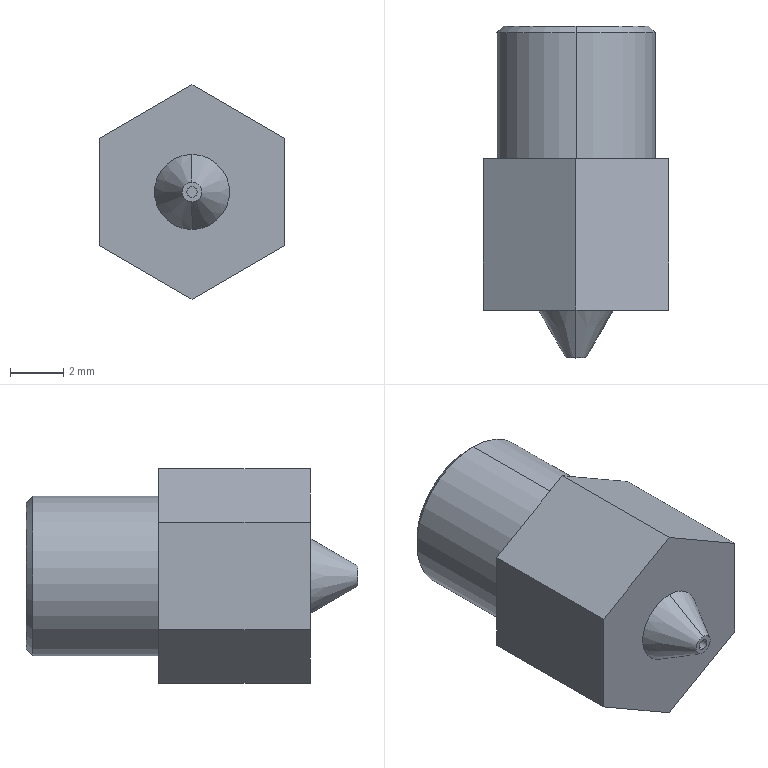Part | SolidWorks | features ICE 1, Revolution 1 | 1 solid | 28 faces | box 7 x 12.5 x 8.083 mm | volume 370.688 mm3 | plane 12 | cylinder 8 | cone 8 | commonest cylinder face diameters 0.4 x2 1 x2 2 x2 6 x2
STEP:
#1=CARTESIAN_POINT('',(0.,12.,1.));
#2=VERTEX_POINT('',#1);
#3=CARTESIAN_POINT('',(0.,12.,-1.));
#4=VERTEX_POINT('',#3);
#5=CARTESIAN_POINT('',(0.,12.,0.));
#6=DIRECTION('',(0.,-1.,0.));
#7=DIRECTION('',(0.,0.,-1.));
#8=AXIS2_PLACEMENT_3D('',#5,#6,#7);
#9=CIRCLE('',#8,1.);
#10=EDGE_CURVE('',#2,#4,#9,.T.);
#11=ORIENTED_EDGE('',*,*,#10,.F.);
#12=CARTESIAN_POINT('',(0.,7.5,1.));
#13=VERTEX_POINT('',#12);
#14=CARTESIAN_POINT('',(0.,0.,1.));
#15=DIRECTION('',(0.,-1.,0.));
#16=VECTOR('',#15,1000.);
#17=LINE('',#14,#16);
#18=EDGE_CURVE('',#2,#13,#17,.T.);
#19=ORIENTED_EDGE('',*,*,#18,.T.);
#20=CARTESIAN_POINT('',(0.,7.5,-1.));
#21=VERTEX_POINT('',#20);
#22=CARTESIAN_POINT('',(0.,7.5,0.));
#23=DIRECTION('',(0.,1.,0.));
#24=DIRECTION('',(0.,0.,1.));
#25=AXIS2_PLACEMENT_3D('',#22,#23,#24);
#26=CIRCLE('',#25,1.);
#27=EDGE_CURVE('',#21,#13,#26,.T.);
#28=ORIENTED_EDGE('',*,*,#27,.F.);
#29=CARTESIAN_POINT('',(0.,0.,-1.));
#30=DIRECTION('',(0.,-1.,0.));
#31=VECTOR('',#30,1000.);
#32=LINE('',#29,#31);
#33=EDGE_CURVE('',#4,#21,#32,.T.);
#34=ORIENTED_EDGE('',*,*,#33,.F.);
#35=EDGE_LOOP('',(#11,#19,#28,#34));
#36=FACE_OUTER_BOUND('',#35,.T.);
#37=CARTESIAN_POINT('',(0.,0.,0.));
#38=DIRECTION('',(0.,-1.,0.));
#39=DIRECTION('',(0.,0.,-1.));
#40=AXIS2_PLACEMENT_3D('',#37,#38,#39);
#41=CYLINDRICAL_SURFACE('',#40,1.);
#42=ADVANCED_FACE('',(#36),#41,.F.);
#43=ORIENTED_EDGE('',*,*,#10,.T.);
#44=CARTESIAN_POINT('',(0.,12.5,-1.289));
#45=VERTEX_POINT('',#44);
#46=CARTESIAN_POINT('',(0.,12.5,-1.289));
#47=DIRECTION('',(0.,0.866,-0.5));
#48=VECTOR('',#47,1000.);
#49=LINE('',#46,#48);
#50=EDGE_CURVE('',#4,#45,#49,.T.);
#51=ORIENTED_EDGE('',*,*,#50,.T.);
#52=CARTESIAN_POINT('',(0.,12.5,1.289));
#53=VERTEX_POINT('',#52);
#54=CARTESIAN_POINT('',(0.,12.5,0.));
#55=DIRECTION('',(0.,-1.,0.));
#56=DIRECTION('',(0.,0.,-1.));
#57=AXIS2_PLACEMENT_3D('',#54,#55,#56);
#58=CIRCLE('',#57,1.289);
#59=EDGE_CURVE('',#53,#45,#58,.T.);
#60=ORIENTED_EDGE('',*,*,#59,.F.);
#61=CARTESIAN_POINT('',(0.,12.5,1.289));
#62=DIRECTION('',(0.,0.866,0.5));
#63=VECTOR('',#62,1000.);
#64=LINE('',#61,#63);
#65=EDGE_CURVE('',#2,#53,#64,.T.);
#66=ORIENTED_EDGE('',*,*,#65,.F.);
#67=EDGE_LOOP('',(#43,#51,#60,#66));
#68=FACE_OUTER_BOUND('',#67,.T.);
#69=CARTESIAN_POINT('',(0.,12.5,0.));
#70=DIRECTION('',(0.,1.,0.));
#71=DIRECTION('',(0.,0.,1.));
#72=AXIS2_PLACEMENT_3D('',#69,#70,#71);
#73=CONICAL_SURFACE('',#72,1.289,0.5236);
#74=ADVANCED_FACE('',(#68),#73,.F.);
#75=CARTESIAN_POINT('',(0.,12.25,-3.));
#76=VERTEX_POINT('',#75);
#77=CARTESIAN_POINT('',(0.,12.25,3.));
#78=VERTEX_POINT('',#77);
#79=CARTESIAN_POINT('',(0.,12.25,0.));
#80=DIRECTION('',(0.,-1.,0.));
#81=DIRECTION('',(0.,0.,-1.));
#82=AXIS2_PLACEMENT_3D('',#79,#80,#81);
#83=CIRCLE('',#82,3.);
#84=EDGE_CURVE('',#76,#78,#83,.T.);
#85=ORIENTED_EDGE('',*,*,#84,.T.);
#86=CARTESIAN_POINT('',(0.,7.5,3.));
#87=VERTEX_POINT('',#86);
#88=CARTESIAN_POINT('',(0.,0.,3.));
#89=DIRECTION('',(0.,-1.,0.));
#90=VECTOR('',#89,1000.);
#91=LINE('',#88,#90);
#92=EDGE_CURVE('',#78,#87,#91,.T.);
#93=ORIENTED_EDGE('',*,*,#92,.T.);
#94=CARTESIAN_POINT('',(0.,7.5,-3.));
#95=VERTEX_POINT('',#94);
#96=CARTESIAN_POINT('',(0.,7.5,0.));
#97=DIRECTION('',(0.,-1.,0.));
#98=DIRECTION('',(0.,0.,1.));
#99=AXIS2_PLACEMENT_3D('',#96,#97,#98);
#100=CIRCLE('',#99,3.);
#101=EDGE_CURVE('',#95,#87,#100,.T.);
#102=ORIENTED_EDGE('',*,*,#101,.F.);
#103=CARTESIAN_POINT('',(0.,0.,-3.));
#104=DIRECTION('',(0.,-1.,0.));
#105=VECTOR('',#104,1000.);
#106=LINE('',#103,#105);
#107=EDGE_CURVE('',#76,#95,#106,.T.);
#108=ORIENTED_EDGE('',*,*,#107,.F.);
#109=EDGE_LOOP('',(#85,#93,#102,#108));
#110=FACE_OUTER_BOUND('',#109,.T.);
#111=CARTESIAN_POINT('',(0.,0.,0.));
#112=DIRECTION('',(0.,-1.,0.));
#113=DIRECTION('',(0.,0.,-1.));
#114=AXIS2_PLACEMENT_3D('',#111,#112,#113);
#115=CYLINDRICAL_SURFACE('',#114,3.);
#116=ADVANCED_FACE('',(#110),#115,.T.);
#117=CARTESIAN_POINT('',(0.,12.5,-2.75));
#118=VERTEX_POINT('',#117);
#119=CARTESIAN_POINT('',(0.,12.5,2.75));
#120=VERTEX_POINT('',#119);
#121=CARTESIAN_POINT('',(0.,12.5,0.));
#122=DIRECTION('',(0.,-1.,0.));
#123=DIRECTION('',(0.,0.,-1.));
#124=AXIS2_PLACEMENT_3D('',#121,#122,#123);
#125=CIRCLE('',#124,2.75);
#126=EDGE_CURVE('',#118,#120,#125,.T.);
#127=ORIENTED_EDGE('',*,*,#126,.T.);
#128=CARTESIAN_POINT('',(0.,12.25,3.));
#129=DIRECTION('',(0.,-0.7071,0.7071));
#130=VECTOR('',#129,1000.);
#131=LINE('',#128,#130);
#132=EDGE_CURVE('',#120,#78,#131,.T.);
#133=ORIENTED_EDGE('',*,*,#132,.T.);
#134=ORIENTED_EDGE('',*,*,#84,.F.);
#135=CARTESIAN_POINT('',(0.,12.25,-3.));
#136=DIRECTION('',(0.,-0.7071,-0.7071));
#137=VECTOR('',#136,1000.);
#138=LINE('',#135,#137);
#139=EDGE_CURVE('',#118,#76,#138,.T.);
#140=ORIENTED_EDGE('',*,*,#139,.F.);
#141=EDGE_LOOP('',(#127,#133,#134,#140));
#142=FACE_OUTER_BOUND('',#141,.T.);
#143=CARTESIAN_POINT('',(0.,12.25,0.));
#144=DIRECTION('',(0.,-1.,0.));
#145=DIRECTION('',(0.,0.,-1.));
#146=AXIS2_PLACEMENT_3D('',#143,#144,#145);
#147=CONICAL_SURFACE('',#146,3.,0.7854);
#148=ADVANCED_FACE('',(#142),#147,.T.);
#149=CARTESIAN_POINT('',(0.,0.6,0.2));
#150=VERTEX_POINT('',#149);
#151=CARTESIAN_POINT('',(0.,0.6,-0.2));
#152=VERTEX_POINT('',#151);
#153=CARTESIAN_POINT('',(0.,0.6,0.));
#154=DIRECTION('',(0.,-1.,0.));
#155=DIRECTION('',(0.,0.,-1.));
#156=AXIS2_PLACEMENT_3D('',#153,#154,#155);
#157=CIRCLE('',#156,0.2);
#158=EDGE_CURVE('',#150,#152,#157,.T.);
#159=ORIENTED_EDGE('',*,*,#158,.F.);
#160=CARTESIAN_POINT('',(0.,0.,0.2));
#161=VERTEX_POINT('',#160);
#162=CARTESIAN_POINT('',(0.,0.,0.2));
#163=DIRECTION('',(0.,-1.,0.));
#164=VECTOR('',#163,1000.);
#165=LINE('',#162,#164);
#166=EDGE_CURVE('',#150,#161,#165,.T.);
#167=ORIENTED_EDGE('',*,*,#166,.T.);
#168=CARTESIAN_POINT('',(0.,0.,-0.2));
#169=VERTEX_POINT('',#168);
#170=CARTESIAN_POINT('',(0.,0.,0.));
#171=DIRECTION('',(0.,-1.,0.));
#172=DIRECTION('',(0.,0.,-1.));
#173=AXIS2_PLACEMENT_3D('',#170,#171,#172);
#174=CIRCLE('',#173,0.2);
#175=EDGE_CURVE('',#161,#169,#174,.T.);
#176=ORIENTED_EDGE('',*,*,#175,.T.);
#177=CARTESIAN_POINT('',(0.,0.,-0.2));
#178=DIRECTION('',(0.,-1.,0.));
#179=VECTOR('',#178,1000.);
#180=LINE('',#177,#179);
#181=EDGE_CURVE('',#152,#169,#180,.T.);
#182=ORIENTED_EDGE('',*,*,#181,.F.);
#183=EDGE_LOOP('',(#159,#167,#176,#182));
#184=FACE_OUTER_BOUND('',#183,.T.);
#185=CARTESIAN_POINT('',(0.,0.,0.));
#186=DIRECTION('',(0.,-1.,0.));
#187=DIRECTION('',(0.,0.,-1.));
#188=AXIS2_PLACEMENT_3D('',#185,#186,#187);
#189=CYLINDRICAL_SURFACE('',#188,0.2);
#190=ADVANCED_FACE('',(#184),#189,.F.);
#191=ORIENTED_EDGE('',*,*,#158,.T.);
#192=CARTESIAN_POINT('',(0.,1.12,-0.5));
#193=VERTEX_POINT('',#192);
#194=CARTESIAN_POINT('',(0.,1.12,-0.5));
#195=DIRECTION('',(0.,0.866,-0.5));
#196=VECTOR('',#195,1000.);
#197=LINE('',#194,#196);
#198=EDGE_CURVE('',#152,#193,#197,.T.);
#199=ORIENTED_EDGE('',*,*,#198,.T.);
#200=CARTESIAN_POINT('',(0.,1.12,0.5));
#201=VERTEX_POINT('',#200);
#202=CARTESIAN_POINT('',(0.,1.12,0.));
#203=DIRECTION('',(0.,-1.,0.));
#204=DIRECTION('',(0.,0.,-1.));
#205=AXIS2_PLACEMENT_3D('',#202,#203,#204);
#206=CIRCLE('',#205,0.5);
#207=EDGE_CURVE('',#201,#193,#206,.T.);
#208=ORIENTED_EDGE('',*,*,#207,.F.);
#209=CARTESIAN_POINT('',(0.,1.12,0.5));
#210=DIRECTION('',(0.,0.866,0.5));
#211=VECTOR('',#210,1000.);
#212=LINE('',#209,#211);
#213=EDGE_CURVE('',#150,#201,#212,.T.);
#214=ORIENTED_EDGE('',*,*,#213,.F.);
#215=EDGE_LOOP('',(#191,#199,#208,#214));
#216=FACE_OUTER_BOUND('',#215,.T.);
#217=CARTESIAN_POINT('',(0.,1.12,0.));
#218=DIRECTION('',(0.,1.,0.));
#219=DIRECTION('',(0.,0.,1.));
#220=AXIS2_PLACEMENT_3D('',#217,#218,#219);
#221=CONICAL_SURFACE('',#220,0.5,0.5236);
#222=ADVANCED_FACE('',(#216),#221,.F.);
#223=CARTESIAN_POINT('',(0.,1.8,0.5));
#224=VERTEX_POINT('',#223);
#225=CARTESIAN_POINT('',(0.,1.8,-0.5));
#226=VERTEX_POINT('',#225);
#227=CARTESIAN_POINT('',(0.,1.8,0.));
#228=DIRECTION('',(0.,-1.,0.));
#229=DIRECTION('',(0.,0.,-1.));
#230=AXIS2_PLACEMENT_3D('',#227,#228,#229);
#231=CIRCLE('',#230,0.5);
#232=EDGE_CURVE('',#224,#226,#231,.T.);
#233=ORIENTED_EDGE('',*,*,#232,.F.);
#234=CARTESIAN_POINT('',(0.,0.,0.5));
#235=DIRECTION('',(0.,-1.,0.));
#236=VECTOR('',#235,1000.);
#237=LINE('',#234,#236);
#238=EDGE_CURVE('',#224,#201,#237,.T.);
#239=ORIENTED_EDGE('',*,*,#238,.T.);
#240=ORIENTED_EDGE('',*,*,#207,.T.);
#241=CARTESIAN_POINT('',(0.,0.,-0.5));
#242=DIRECTION('',(0.,-1.,0.));
#243=VECTOR('',#242,1000.);
#244=LINE('',#241,#243);
#245=EDGE_CURVE('',#226,#193,#244,.T.);
#246=ORIENTED_EDGE('',*,*,#245,.F.);
#247=EDGE_LOOP('',(#233,#239,#240,#246));
#248=FACE_OUTER_BOUND('',#247,.T.);
#249=CARTESIAN_POINT('',(0.,0.,0.));
#250=DIRECTION('',(0.,-1.,0.));
#251=DIRECTION('',(0.,0.,-1.));
#252=AXIS2_PLACEMENT_3D('',#249,#250,#251);
#253=CYLINDRICAL_SURFACE('',#252,0.5);
#254=ADVANCED_FACE('',(#248),#253,.F.);
#255=CARTESIAN_POINT('',(0.,0.,-0.375));
#256=VERTEX_POINT('',#255);
#257=CARTESIAN_POINT('',(0.,0.,0.375));
#258=VERTEX_POINT('',#257);
#259=CARTESIAN_POINT('',(0.,0.,0.));
#260=DIRECTION('',(0.,-1.,0.));
#261=DIRECTION('',(0.,0.,-1.));
#262=AXIS2_PLACEMENT_3D('',#259,#260,#261);
#263=CIRCLE('',#262,0.375);
#264=EDGE_CURVE('',#256,#258,#263,.T.);
#265=ORIENTED_EDGE('',*,*,#264,.F.);
#266=CARTESIAN_POINT('',(0.,1.8,-1.414));
#267=VERTEX_POINT('',#266);
#268=CARTESIAN_POINT('',(0.,0.,-0.375));
#269=DIRECTION('',(0.,0.866,-0.5));
#270=VECTOR('',#269,1000.);
#271=LINE('',#268,#270);
#272=EDGE_CURVE('',#256,#267,#271,.T.);
#273=ORIENTED_EDGE('',*,*,#272,.T.);
#274=CARTESIAN_POINT('',(0.,1.8,1.414));
#275=VERTEX_POINT('',#274);
#276=CARTESIAN_POINT('',(0.,1.8,0.));
#277=DIRECTION('',(0.,-1.,0.));
#278=DIRECTION('',(0.,0.,-1.));
#279=AXIS2_PLACEMENT_3D('',#276,#277,#278);
#280=CIRCLE('',#279,1.414);
#281=EDGE_CURVE('',#267,#275,#280,.T.);
#282=ORIENTED_EDGE('',*,*,#281,.T.);
#283=CARTESIAN_POINT('',(0.,0.,0.375));
#284=DIRECTION('',(0.,0.866,0.5));
#285=VECTOR('',#284,1000.);
#286=LINE('',#283,#285);
#287=EDGE_CURVE('',#258,#275,#286,.T.);
#288=ORIENTED_EDGE('',*,*,#287,.F.);
#289=EDGE_LOOP('',(#265,#273,#282,#288));
#290=FACE_OUTER_BOUND('',#289,.T.);
#291=CARTESIAN_POINT('',(0.,0.,0.));
#292=DIRECTION('',(0.,1.,0.));
#293=DIRECTION('',(0.,0.,1.));
#294=AXIS2_PLACEMENT_3D('',#291,#292,#293);
#295=CONICAL_SURFACE('',#294,0.375,0.5236);
#296=ADVANCED_FACE('',(#290),#295,.T.);
#297=ORIENTED_EDGE('',*,*,#272,.F.);
#298=CARTESIAN_POINT('',(0.,0.,0.));
#299=DIRECTION('',(0.,-1.,0.));
#300=DIRECTION('',(0.,0.,-1.));
#301=AXIS2_PLACEMENT_3D('',#298,#299,#300);
#302=CIRCLE('',#301,0.375);
#303=EDGE_CURVE('',#258,#256,#302,.T.);
#304=ORIENTED_EDGE('',*,*,#303,.F.);
#305=ORIENTED_EDGE('',*,*,#287,.T.);
#306=CARTESIAN_POINT('',(0.,1.8,0.));
#307=DIRECTION('',(0.,-1.,0.));
#308=DIRECTION('',(0.,0.,-1.));
#309=AXIS2_PLACEMENT_3D('',#306,#307,#308);
#310=CIRCLE('',#309,1.414);
#311=EDGE_CURVE('',#275,#267,#310,.T.);
#312=ORIENTED_EDGE('',*,*,#311,.T.);
#313=EDGE_LOOP('',(#297,#304,#305,#312));
#314=FACE_OUTER_BOUND('',#313,.T.);
#315=CARTESIAN_POINT('',(0.,0.,0.));
#316=DIRECTION('',(0.,1.,0.));
#317=DIRECTION('',(0.,0.,1.));
#318=AXIS2_PLACEMENT_3D('',#315,#316,#317);
#319=CONICAL_SURFACE('',#318,0.375,0.5236);
#320=ADVANCED_FACE('',(#314),#319,.T.);
#321=ORIENTED_EDGE('',*,*,#311,.F.);
#322=ORIENTED_EDGE('',*,*,#281,.F.);
#323=EDGE_LOOP('',(#321,#322));
#324=FACE_BOUND('',#323,.T.);
#325=CARTESIAN_POINT('',(3.5,1.8,2.021));
#326=VERTEX_POINT('',#325);
#327=CARTESIAN_POINT('',(0.,1.8,4.041));
#328=VERTEX_POINT('',#327);
#329=CARTESIAN_POINT('',(3.5,1.8,2.021));
#330=DIRECTION('',(-0.866,0.,0.5));
#331=VECTOR('',#330,1000.);
#332=LINE('',#329,#331);
#333=EDGE_CURVE('',#326,#328,#332,.T.);
#334=ORIENTED_EDGE('',*,*,#333,.T.);
#335=CARTESIAN_POINT('',(-3.5,1.8,2.021));
#336=VERTEX_POINT('',#335);
#337=CARTESIAN_POINT('',(0.,1.8,4.041));
#338=DIRECTION('',(-0.866,0.,-0.5));
#339=VECTOR('',#338,1000.);
#340=LINE('',#337,#339);
#341=EDGE_CURVE('',#328,#336,#340,.T.);
#342=ORIENTED_EDGE('',*,*,#341,.T.);
#343=CARTESIAN_POINT('',(-3.5,1.8,-2.021));
#344=VERTEX_POINT('',#343);
#345=CARTESIAN_POINT('',(-3.5,1.8,2.021));
#346=DIRECTION('',(0.,0.,-1.));
#347=VECTOR('',#346,1000.);
#348=LINE('',#345,#347);
#349=EDGE_CURVE('',#336,#344,#348,.T.);
#350=ORIENTED_EDGE('',*,*,#349,.T.);
#351=CARTESIAN_POINT('',(0.,1.8,-4.041));
#352=VERTEX_POINT('',#351);
#353=CARTESIAN_POINT('',(-3.5,1.8,-2.021));
#354=DIRECTION('',(0.866,0.,-0.5));
#355=VECTOR('',#354,1000.);
#356=LINE('',#353,#355);
#357=EDGE_CURVE('',#344,#352,#356,.T.);
#358=ORIENTED_EDGE('',*,*,#357,.T.);
#359=CARTESIAN_POINT('',(3.5,1.8,-2.021));
#360=VERTEX_POINT('',#359);
#361=CARTESIAN_POINT('',(0.,1.8,-4.041));
#362=DIRECTION('',(0.866,0.,0.5));
#363=VECTOR('',#362,1000.);
#364=LINE('',#361,#363);
#365=EDGE_CURVE('',#352,#360,#364,.T.);
#366=ORIENTED_EDGE('',*,*,#365,.T.);
#367=CARTESIAN_POINT('',(3.5,1.8,-2.021));
#368=DIRECTION('',(0.,0.,1.));
#369=VECTOR('',#368,1000.);
#370=LINE('',#367,#369);
#371=EDGE_CURVE('',#360,#326,#370,.T.);
#372=ORIENTED_EDGE('',*,*,#371,.T.);
#373=EDGE_LOOP('',(#334,#342,#350,#358,#366,#372));
#374=FACE_OUTER_BOUND('',#373,.T.);
#375=CARTESIAN_POINT('',(1.414,1.8,0.));
#376=DIRECTION('',(0.,-1.,0.));
#377=DIRECTION('',(0.,0.,-1.));
#378=AXIS2_PLACEMENT_3D('',#375,#376,#377);
#379=PLANE('',#378);
#380=ADVANCED_FACE('',(#324,#374),#379,.T.);
#381=ORIENTED_EDGE('',*,*,#238,.F.);
#382=CARTESIAN_POINT('',(0.,1.8,0.));
#383=DIRECTION('',(0.,-1.,0.));
#384=DIRECTION('',(0.,0.,-1.));
#385=AXIS2_PLACEMENT_3D('',#382,#383,#384);
#386=CIRCLE('',#385,0.5);
#387=EDGE_CURVE('',#226,#224,#386,.T.);
#388=ORIENTED_EDGE('',*,*,#387,.F.);
#389=ORIENTED_EDGE('',*,*,#245,.T.);
#390=CARTESIAN_POINT('',(0.,1.12,0.));
#391=DIRECTION('',(0.,-1.,0.));
#392=DIRECTION('',(0.,0.,-1.));
#393=AXIS2_PLACEMENT_3D('',#390,#391,#392);
#394=CIRCLE('',#393,0.5);
#395=EDGE_CURVE('',#193,#201,#394,.T.);
#396=ORIENTED_EDGE('',*,*,#395,.T.);
#397=EDGE_LOOP('',(#381,#388,#389,#396));
#398=FACE_OUTER_BOUND('',#397,.T.);
#399=CARTESIAN_POINT('',(0.,0.,0.));
#400=DIRECTION('',(0.,-1.,0.));
#401=DIRECTION('',(0.,0.,-1.));
#402=AXIS2_PLACEMENT_3D('',#399,#400,#401);
#403=CYLINDRICAL_SURFACE('',#402,0.5);
#404=ADVANCED_FACE('',(#398),#403,.F.);
#405=ORIENTED_EDGE('',*,*,#198,.F.);
#406=CARTESIAN_POINT('',(0.,0.6,0.));
#407=DIRECTION('',(0.,-1.,0.));
#408=DIRECTION('',(0.,0.,-1.));
#409=AXIS2_PLACEMENT_3D('',#406,#407,#408);
#410=CIRCLE('',#409,0.2);
#411=EDGE_CURVE('',#152,#150,#410,.T.);
#412=ORIENTED_EDGE('',*,*,#411,.T.);
#413=ORIENTED_EDGE('',*,*,#213,.T.);
#414=ORIENTED_EDGE('',*,*,#395,.F.);
#415=EDGE_LOOP('',(#405,#412,#413,#414));
#416=FACE_OUTER_BOUND('',#415,.T.);
#417=CARTESIAN_POINT('',(0.,1.12,0.));
#418=DIRECTION('',(0.,1.,0.));
#419=DIRECTION('',(0.,0.,1.));
#420=AXIS2_PLACEMENT_3D('',#417,#418,#419);
#421=CONICAL_SURFACE('',#420,0.5,0.5236);
#422=ADVANCED_FACE('',(#416),#421,.F.);
#423=ORIENTED_EDGE('',*,*,#166,.F.);
#424=ORIENTED_EDGE('',*,*,#411,.F.);
#425=ORIENTED_EDGE('',*,*,#181,.T.);
#426=CARTESIAN_POINT('',(0.,0.,0.));
#427=DIRECTION('',(0.,-1.,0.));
#428=DIRECTION('',(0.,0.,-1.));
#429=AXIS2_PLACEMENT_3D('',#426,#427,#428);
#430=CIRCLE('',#429,0.2);
#431=EDGE_CURVE('',#169,#161,#430,.T.);
#432=ORIENTED_EDGE('',*,*,#431,.T.);
#433=EDGE_LOOP('',(#423,#424,#425,#432));
#434=FACE_OUTER_BOUND('',#433,.T.);
#435=CARTESIAN_POINT('',(0.,0.,0.));
#436=DIRECTION('',(0.,-1.,0.));
#437=DIRECTION('',(0.,0.,-1.));
#438=AXIS2_PLACEMENT_3D('',#435,#436,#437);
#439=CYLINDRICAL_SURFACE('',#438,0.2);
#440=ADVANCED_FACE('',(#434),#439,.F.);
#441=ORIENTED_EDGE('',*,*,#303,.T.);
#442=ORIENTED_EDGE('',*,*,#264,.T.);
#443=EDGE_LOOP('',(#441,#442));
#444=FACE_OUTER_BOUND('',#443,.T.);
#445=ORIENTED_EDGE('',*,*,#431,.F.);
#446=ORIENTED_EDGE('',*,*,#175,.F.);
#447=EDGE_LOOP('',(#445,#446));
#448=FACE_BOUND('',#447,.T.);
#449=CARTESIAN_POINT('',(0.2,0.,0.));
#450=DIRECTION('',(0.,-1.,0.));
#451=DIRECTION('',(0.,0.,-1.));
#452=AXIS2_PLACEMENT_3D('',#449,#450,#451);
#453=PLANE('',#452);
#454=ADVANCED_FACE('',(#444,#448),#453,.T.);
#455=ORIENTED_EDGE('',*,*,#387,.T.);
#456=ORIENTED_EDGE('',*,*,#232,.T.);
#457=EDGE_LOOP('',(#455,#456));
#458=FACE_OUTER_BOUND('',#457,.T.);
#459=CARTESIAN_POINT('',(0.,1.8,0.));
#460=DIRECTION('',(0.,-1.,0.));
#461=DIRECTION('',(0.,0.,-1.));
#462=AXIS2_PLACEMENT_3D('',#459,#460,#461);
#463=PLANE('',#462);
#464=ADVANCED_FACE('',(#458),#463,.T.);
#465=ORIENTED_EDGE('',*,*,#101,.T.);
#466=CARTESIAN_POINT('',(0.,7.5,0.));
#467=DIRECTION('',(0.,-1.,0.));
#468=DIRECTION('',(0.,0.,1.));
#469=AXIS2_PLACEMENT_3D('',#466,#467,#468);
#470=CIRCLE('',#469,3.);
#471=EDGE_CURVE('',#87,#95,#470,.T.);
#472=ORIENTED_EDGE('',*,*,#471,.T.);
#473=EDGE_LOOP('',(#465,#472));
#474=FACE_BOUND('',#473,.T.);
#475=CARTESIAN_POINT('',(3.5,7.5,2.021));
#476=VERTEX_POINT('',#475);
#477=CARTESIAN_POINT('',(0.,7.5,4.041));
#478=VERTEX_POINT('',#477);
#479=CARTESIAN_POINT('',(3.5,7.5,2.021));
#480=DIRECTION('',(-0.866,0.,0.5));
#481=VECTOR('',#480,1000.);
#482=LINE('',#479,#481);
#483=EDGE_CURVE('',#476,#478,#482,.T.);
#484=ORIENTED_EDGE('',*,*,#483,.F.);
#485=CARTESIAN_POINT('',(3.5,7.5,-2.021));
#486=VERTEX_POINT('',#485);
#487=CARTESIAN_POINT('',(3.5,7.5,-2.021));
#488=DIRECTION('',(0.,0.,1.));
#489=VECTOR('',#488,1000.);
#490=LINE('',#487,#489);
#491=EDGE_CURVE('',#486,#476,#490,.T.);
#492=ORIENTED_EDGE('',*,*,#491,.F.);
#493=CARTESIAN_POINT('',(0.,7.5,-4.041));
#494=VERTEX_POINT('',#493);
#495=CARTESIAN_POINT('',(0.,7.5,-4.041));
#496=DIRECTION('',(0.866,0.,0.5));
#497=VECTOR('',#496,1000.);
#498=LINE('',#495,#497);
#499=EDGE_CURVE('',#494,#486,#498,.T.);
#500=ORIENTED_EDGE('',*,*,#499,.F.);
#501=CARTESIAN_POINT('',(-3.5,7.5,-2.021));
#502=VERTEX_POINT('',#501);
#503=CARTESIAN_POINT('',(-3.5,7.5,-2.021));
#504=DIRECTION('',(0.866,0.,-0.5));
#505=VECTOR('',#504,1000.);
#506=LINE('',#503,#505);
#507=EDGE_CURVE('',#502,#494,#506,.T.);
#508=ORIENTED_EDGE('',*,*,#507,.F.);
#509=CARTESIAN_POINT('',(-3.5,7.5,2.021));
#510=VERTEX_POINT('',#509);
#511=CARTESIAN_POINT('',(-3.5,7.5,2.021));
#512=DIRECTION('',(0.,0.,-1.));
#513=VECTOR('',#512,1000.);
#514=LINE('',#511,#513);
#515=EDGE_CURVE('',#510,#502,#514,.T.);
#516=ORIENTED_EDGE('',*,*,#515,.F.);
#517=CARTESIAN_POINT('',(0.,7.5,4.041));
#518=DIRECTION('',(-0.866,0.,-0.5));
#519=VECTOR('',#518,1000.);
#520=LINE('',#517,#519);
#521=EDGE_CURVE('',#478,#510,#520,.T.);
#522=ORIENTED_EDGE('',*,*,#521,.F.);
#523=EDGE_LOOP('',(#484,#492,#500,#508,#516,#522));
#524=FACE_OUTER_BOUND('',#523,.T.);
#525=CARTESIAN_POINT('',(2.75,7.5,0.));
#526=DIRECTION('',(0.,1.,0.));
#527=DIRECTION('',(0.,0.,1.));
#528=AXIS2_PLACEMENT_3D('',#525,#526,#527);
#529=PLANE('',#528);
#530=ADVANCED_FACE('',(#474,#524),#529,.T.);
#531=CARTESIAN_POINT('',(0.,23.193,4.041));
#532=DIRECTION('',(0.,-1.,0.));
#533=VECTOR('',#532,1000.);
#534=LINE('',#531,#533);
#535=EDGE_CURVE('',#478,#328,#534,.T.);
#536=ORIENTED_EDGE('',*,*,#535,.F.);
#537=ORIENTED_EDGE('',*,*,#521,.T.);
#538=CARTESIAN_POINT('',(-3.5,23.193,2.021));
#539=DIRECTION('',(0.,-1.,0.));
#540=VECTOR('',#539,1000.);
#541=LINE('',#538,#540);
#542=EDGE_CURVE('',#510,#336,#541,.T.);
#543=ORIENTED_EDGE('',*,*,#542,.T.);
#544=ORIENTED_EDGE('',*,*,#341,.F.);
#545=EDGE_LOOP('',(#536,#537,#543,#544));
#546=FACE_OUTER_BOUND('',#545,.T.);
#547=CARTESIAN_POINT('',(0.,23.193,4.041));
#548=DIRECTION('',(-0.5,0.,0.866));
#549=DIRECTION('',(0.866,0.,0.5));
#550=AXIS2_PLACEMENT_3D('',#547,#548,#549);
#551=PLANE('',#550);
#552=ADVANCED_FACE('',(#546),#551,.T.);
#553=ORIENTED_EDGE('',*,*,#542,.F.);
#554=ORIENTED_EDGE('',*,*,#515,.T.);
#555=CARTESIAN_POINT('',(-3.5,23.193,-2.021));
#556=DIRECTION('',(0.,-1.,0.));
#557=VECTOR('',#556,1000.);
#558=LINE('',#555,#557);
#559=EDGE_CURVE('',#502,#344,#558,.T.);
#560=ORIENTED_EDGE('',*,*,#559,.T.);
#561=ORIENTED_EDGE('',*,*,#349,.F.);
#562=EDGE_LOOP('',(#553,#554,#560,#561));
#563=FACE_OUTER_BOUND('',#562,.T.);
#564=CARTESIAN_POINT('',(-3.5,23.193,2.021));
#565=DIRECTION('',(-1.,0.,0.));
#566=DIRECTION('',(0.,0.,1.));
#567=AXIS2_PLACEMENT_3D('',#564,#565,#566);
#568=PLANE('',#567);
#569=ADVANCED_FACE('',(#563),#568,.T.);
#570=ORIENTED_EDGE('',*,*,#559,.F.);
#571=ORIENTED_EDGE('',*,*,#507,.T.);
#572=CARTESIAN_POINT('',(0.,23.193,-4.041));
#573=DIRECTION('',(0.,-1.,0.));
#574=VECTOR('',#573,1000.);
#575=LINE('',#572,#574);
#576=EDGE_CURVE('',#494,#352,#575,.T.);
#577=ORIENTED_EDGE('',*,*,#576,.T.);
#578=ORIENTED_EDGE('',*,*,#357,.F.);
#579=EDGE_LOOP('',(#570,#571,#577,#578));
#580=FACE_OUTER_BOUND('',#579,.T.);
#581=CARTESIAN_POINT('',(-3.5,23.193,-2.021));
#582=DIRECTION('',(-0.5,0.,-0.866));
#583=DIRECTION('',(-0.866,0.,0.5));
#584=AXIS2_PLACEMENT_3D('',#581,#582,#583);
#585=PLANE('',#584);
#586=ADVANCED_FACE('',(#580),#585,.T.);
#587=ORIENTED_EDGE('',*,*,#576,.F.);
#588=ORIENTED_EDGE('',*,*,#499,.T.);
#589=CARTESIAN_POINT('',(3.5,23.193,-2.021));
#590=DIRECTION('',(0.,-1.,0.));
#591=VECTOR('',#590,1000.);
#592=LINE('',#589,#591);
#593=EDGE_CURVE('',#486,#360,#592,.T.);
#594=ORIENTED_EDGE('',*,*,#593,.T.);
#595=ORIENTED_EDGE('',*,*,#365,.F.);
#596=EDGE_LOOP('',(#587,#588,#594,#595));
#597=FACE_OUTER_BOUND('',#596,.T.);
#598=CARTESIAN_POINT('',(0.,23.193,-4.041));
#599=DIRECTION('',(0.5,0.,-0.866));
#600=DIRECTION('',(-0.866,0.,-0.5));
#601=AXIS2_PLACEMENT_3D('',#598,#599,#600);
#602=PLANE('',#601);
#603=ADVANCED_FACE('',(#597),#602,.T.);
#604=ORIENTED_EDGE('',*,*,#593,.F.);
#605=ORIENTED_EDGE('',*,*,#491,.T.);
#606=CARTESIAN_POINT('',(3.5,23.193,2.021));
#607=DIRECTION('',(0.,-1.,0.));
#608=VECTOR('',#607,1000.);
#609=LINE('',#606,#608);
#610=EDGE_CURVE('',#476,#326,#609,.T.);
#611=ORIENTED_EDGE('',*,*,#610,.T.);
#612=ORIENTED_EDGE('',*,*,#371,.F.);
#613=EDGE_LOOP('',(#604,#605,#611,#612));
#614=FACE_OUTER_BOUND('',#613,.T.);
#615=CARTESIAN_POINT('',(3.5,23.193,-2.021));
#616=DIRECTION('',(1.,0.,0.));
#617=DIRECTION('',(0.,0.,-1.));
#618=AXIS2_PLACEMENT_3D('',#615,#616,#617);
#619=PLANE('',#618);
#620=ADVANCED_FACE('',(#614),#619,.T.);
#621=ORIENTED_EDGE('',*,*,#610,.F.);
#622=ORIENTED_EDGE('',*,*,#483,.T.);
#623=ORIENTED_EDGE('',*,*,#535,.T.);
#624=ORIENTED_EDGE('',*,*,#333,.F.);
#625=EDGE_LOOP('',(#621,#622,#623,#624));
#626=FACE_OUTER_BOUND('',#625,.T.);
#627=CARTESIAN_POINT('',(3.5,23.193,2.021));
#628=DIRECTION('',(0.5,0.,0.866));
#629=DIRECTION('',(0.866,0.,-0.5));
#630=AXIS2_PLACEMENT_3D('',#627,#628,#629);
#631=PLANE('',#630);
#632=ADVANCED_FACE('',(#626),#631,.T.);
#633=ORIENTED_EDGE('',*,*,#132,.F.);
#634=CARTESIAN_POINT('',(0.,12.5,0.));
#635=DIRECTION('',(0.,-1.,0.));
#636=DIRECTION('',(0.,0.,-1.));
#637=AXIS2_PLACEMENT_3D('',#634,#635,#636);
#638=CIRCLE('',#637,2.75);
#639=EDGE_CURVE('',#120,#118,#638,.T.);
#640=ORIENTED_EDGE('',*,*,#639,.T.);
#641=ORIENTED_EDGE('',*,*,#139,.T.);
#642=CARTESIAN_POINT('',(0.,12.25,0.));
#643=DIRECTION('',(0.,-1.,0.));
#644=DIRECTION('',(0.,0.,-1.));
#645=AXIS2_PLACEMENT_3D('',#642,#643,#644);
#646=CIRCLE('',#645,3.);
#647=EDGE_CURVE('',#78,#76,#646,.T.);
#648=ORIENTED_EDGE('',*,*,#647,.F.);
#649=EDGE_LOOP('',(#633,#640,#641,#648));
#650=FACE_OUTER_BOUND('',#649,.T.);
#651=CARTESIAN_POINT('',(0.,12.25,0.));
#652=DIRECTION('',(0.,-1.,0.));
#653=DIRECTION('',(0.,0.,-1.));
#654=AXIS2_PLACEMENT_3D('',#651,#652,#653);
#655=CONICAL_SURFACE('',#654,3.,0.7854);
#656=ADVANCED_FACE('',(#650),#655,.T.);
#657=ORIENTED_EDGE('',*,*,#92,.F.);
#658=ORIENTED_EDGE('',*,*,#647,.T.);
#659=ORIENTED_EDGE('',*,*,#107,.T.);
#660=ORIENTED_EDGE('',*,*,#471,.F.);
#661=EDGE_LOOP('',(#657,#658,#659,#660));
#662=FACE_OUTER_BOUND('',#661,.T.);
#663=CARTESIAN_POINT('',(0.,0.,0.));
#664=DIRECTION('',(0.,-1.,0.));
#665=DIRECTION('',(0.,0.,-1.));
#666=AXIS2_PLACEMENT_3D('',#663,#664,#665);
#667=CYLINDRICAL_SURFACE('',#666,3.);
#668=ADVANCED_FACE('',(#662),#667,.T.);
#669=ORIENTED_EDGE('',*,*,#59,.T.);
#670=CARTESIAN_POINT('',(0.,12.5,0.));
#671=DIRECTION('',(0.,-1.,0.));
#672=DIRECTION('',(0.,0.,-1.));
#673=AXIS2_PLACEMENT_3D('',#670,#671,#672);
#674=CIRCLE('',#673,1.289);
#675=EDGE_CURVE('',#45,#53,#674,.T.);
#676=ORIENTED_EDGE('',*,*,#675,.T.);
#677=EDGE_LOOP('',(#669,#676));
#678=FACE_BOUND('',#677,.T.);
#679=ORIENTED_EDGE('',*,*,#126,.F.);
#680=ORIENTED_EDGE('',*,*,#639,.F.);
#681=EDGE_LOOP('',(#679,#680));
#682=FACE_OUTER_BOUND('',#681,.T.);
#683=CARTESIAN_POINT('',(2.75,12.5,0.));
#684=DIRECTION('',(0.,1.,0.));
#685=DIRECTION('',(0.,0.,1.));
#686=AXIS2_PLACEMENT_3D('',#683,#684,#685);
#687=PLANE('',#686);
#688=ADVANCED_FACE('',(#678,#682),#687,.T.);
#689=ORIENTED_EDGE('',*,*,#50,.F.);
#690=CARTESIAN_POINT('',(0.,12.,0.));
#691=DIRECTION('',(0.,-1.,0.));
#692=DIRECTION('',(0.,0.,-1.));
#693=AXIS2_PLACEMENT_3D('',#690,#691,#692);
#694=CIRCLE('',#693,1.);
#695=EDGE_CURVE('',#4,#2,#694,.T.);
#696=ORIENTED_EDGE('',*,*,#695,.T.);
#697=ORIENTED_EDGE('',*,*,#65,.T.);
#698=ORIENTED_EDGE('',*,*,#675,.F.);
#699=EDGE_LOOP('',(#689,#696,#697,#698));
#700=FACE_OUTER_BOUND('',#699,.T.);
#701=CARTESIAN_POINT('',(0.,12.5,0.));
#702=DIRECTION('',(0.,1.,0.));
#703=DIRECTION('',(0.,0.,1.));
#704=AXIS2_PLACEMENT_3D('',#701,#702,#703);
#705=CONICAL_SURFACE('',#704,1.289,0.5236);
#706=ADVANCED_FACE('',(#700),#705,.F.);
#707=ORIENTED_EDGE('',*,*,#18,.F.);
#708=ORIENTED_EDGE('',*,*,#695,.F.);
#709=ORIENTED_EDGE('',*,*,#33,.T.);
#710=CARTESIAN_POINT('',(0.,7.5,0.));
#711=DIRECTION('',(0.,1.,0.));
#712=DIRECTION('',(0.,0.,1.));
#713=AXIS2_PLACEMENT_3D('',#710,#711,#712);
#714=CIRCLE('',#713,1.);
#715=EDGE_CURVE('',#13,#21,#714,.T.);
#716=ORIENTED_EDGE('',*,*,#715,.F.);
#717=EDGE_LOOP('',(#707,#708,#709,#716));
#718=FACE_OUTER_BOUND('',#717,.T.);
#719=CARTESIAN_POINT('',(0.,0.,0.));
#720=DIRECTION('',(0.,-1.,0.));
#721=DIRECTION('',(0.,0.,-1.));
#722=AXIS2_PLACEMENT_3D('',#719,#720,#721);
#723=CYLINDRICAL_SURFACE('',#722,1.);
#724=ADVANCED_FACE('',(#718),#723,.F.);
#725=ORIENTED_EDGE('',*,*,#27,.T.);
#726=ORIENTED_EDGE('',*,*,#715,.T.);
#727=EDGE_LOOP('',(#725,#726));
#728=FACE_OUTER_BOUND('',#727,.T.);
#729=CARTESIAN_POINT('',(2.75,7.5,0.));
#730=DIRECTION('',(0.,1.,0.));
#731=DIRECTION('',(0.,0.,1.));
#732=AXIS2_PLACEMENT_3D('',#729,#730,#731);
#733=PLANE('',#732);
#734=ADVANCED_FACE('',(#728),#733,.T.);
#735=CLOSED_SHELL('',(#42,#74,#116,#148,#190,#222,#254,#296,#320,#380,#404,#422,#440,#454,#464,#530,#552,#569,#586,#603,#620,#632,#656,#668,#688,#706,#724,#734));
#736=MANIFOLD_SOLID_BREP('',#735);
#737=CARTESIAN_POINT('',(0.,0.,0.));
#738=DIRECTION('',(0.,0.,1.));
#739=DIRECTION('',(1.,0.,0.));
#740=AXIS2_PLACEMENT_3D('',#737,#738,#739);
#741=(LENGTH_UNIT()NAMED_UNIT(*)SI_UNIT(.MILLI.,.METRE.));
#742=UNCERTAINTY_MEASURE_WITH_UNIT(LENGTH_MEASURE(0.00001),#741,'','');
#743=(NAMED_UNIT(*)PLANE_ANGLE_UNIT()SI_UNIT($,.RADIAN.));
#744=(NAMED_UNIT(*)SI_UNIT($,.STERADIAN.)SOLID_ANGLE_UNIT());
#745=(GEOMETRIC_REPRESENTATION_CONTEXT(3)GLOBAL_UNCERTAINTY_ASSIGNED_CONTEXT((#742))GLOBAL_UNIT_ASSIGNED_CONTEXT((#741,#743,#744))REPRESENTATION_CONTEXT('',''));
#746=ADVANCED_BREP_SHAPE_REPRESENTATION('',(#736,#740),#745);